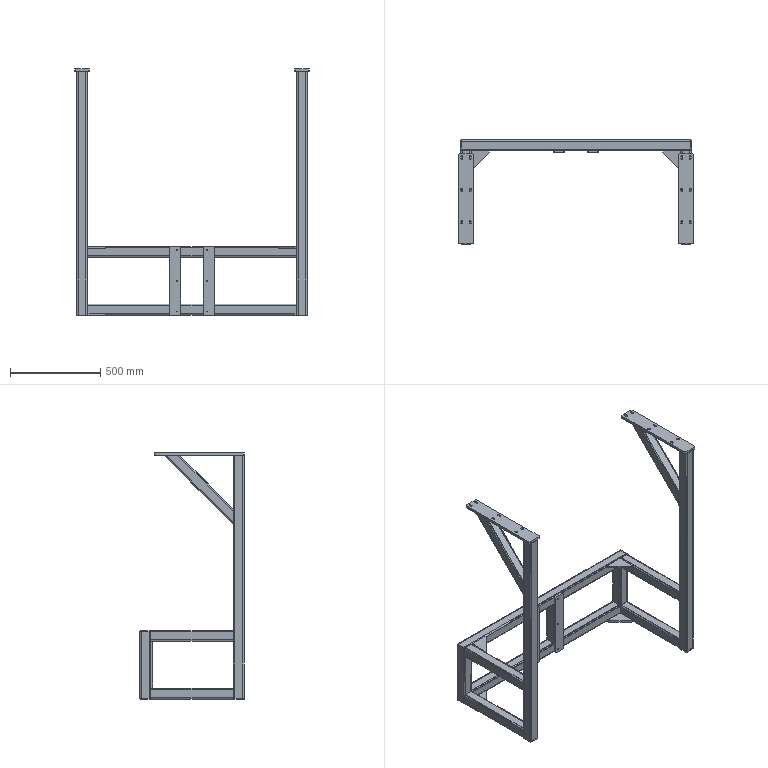Part | SolidWorks | features BaseBody 24 | 24 solids | 424 faces | box 1300 x 580 x 1365 mm | volume 9754704 mm3 | plane 244 | cylinder 168 | cone 12 | commonest cylinder face diameters 8 x64 16 x56 5 x24 11 x24